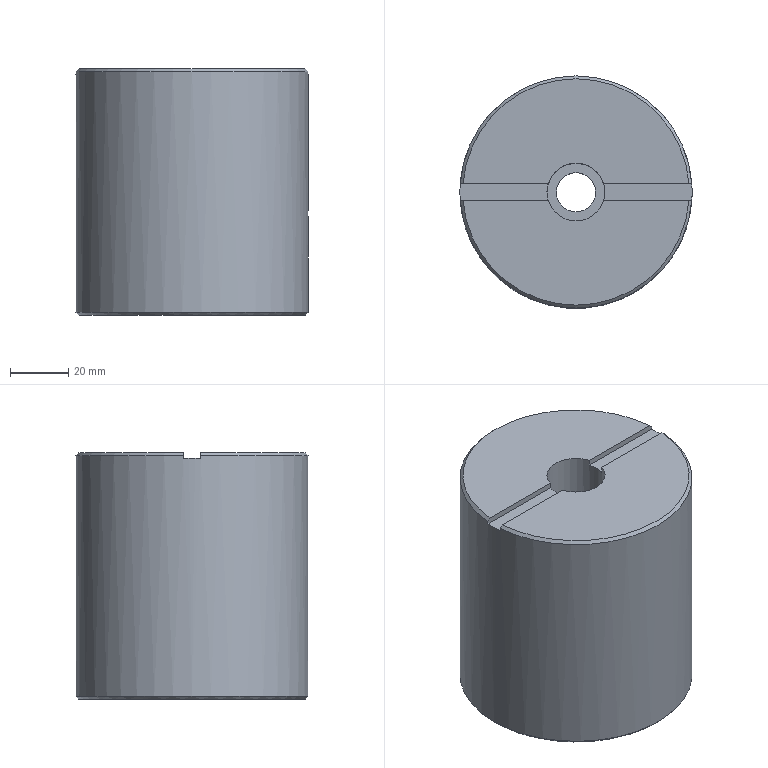Part | STEP file | 008_id4090_x_t | 1 solid | 18 faces | box 80 x 80 x 85 mm | volume 404567 mm3 | plane 11 | cylinder 4 | cone 3 | commonest cylinder face diameters 3.4 x1 13.509 x1 20.008 x1 80 x1
STEP:
#1=CARTESIAN_POINT('',(3931.979,552.,5.));
#2=VERTEX_POINT('',#1);
#3=CARTESIAN_POINT('',(3961.32,552.,5.));
#4=VERTEX_POINT('',#3);
#5=CARTESIAN_POINT('',(3873.935,552.,5.));
#6=DIRECTION('',(1.,0.,0.));
#7=VECTOR('',#6,1.);
#8=LINE('',#5,#7);
#9=EDGE_CURVE('',#2,#4,#8,.T.);
#10=ORIENTED_EDGE('',*,*,#9,.F.);
#11=CARTESIAN_POINT('',(3912.892,552.,5.));
#12=VERTEX_POINT('',#11);
#13=CARTESIAN_POINT('',(3922.435,555.,5.));
#14=DIRECTION('',(0.,0.,-1.));
#15=DIRECTION('',(-1.,0.,0.));
#16=AXIS2_PLACEMENT_3D('',#13,#14,#15);
#17=CIRCLE('',#16,10.004);
#18=EDGE_CURVE('',#2,#12,#17,.T.);
#19=ORIENTED_EDGE('',*,*,#18,.T.);
#20=CARTESIAN_POINT('',(3883.551,552.,5.));
#21=VERTEX_POINT('',#20);
#22=CARTESIAN_POINT('',(3873.935,552.,5.));
#23=DIRECTION('',(1.,0.,0.));
#24=VECTOR('',#23,1.);
#25=LINE('',#22,#24);
#26=EDGE_CURVE('',#21,#12,#25,.T.);
#27=ORIENTED_EDGE('',*,*,#26,.F.);
#28=CARTESIAN_POINT('',(3922.435,555.,5.));
#29=DIRECTION('',(0.,0.,-1.));
#30=DIRECTION('',(1.,0.,0.));
#31=AXIS2_PLACEMENT_3D('',#28,#29,#30);
#32=CIRCLE('',#31,39.);
#33=EDGE_CURVE('',#4,#21,#32,.T.);
#34=ORIENTED_EDGE('',*,*,#33,.F.);
#35=EDGE_LOOP('',(#10,#19,#27,#34));
#36=FACE_OUTER_BOUND('',#35,.T.);
#37=CARTESIAN_POINT('',(3922.435,555.,5.));
#38=DIRECTION('',(0.,0.,1.));
#39=DIRECTION('',(1.,0.,0.));
#40=AXIS2_PLACEMENT_3D('',#37,#38,#39);
#41=PLANE('',#40);
#42=ADVANCED_FACE('',(#36),#41,.T.);
#43=CARTESIAN_POINT('',(3883.551,558.,5.));
#44=VERTEX_POINT('',#43);
#45=CARTESIAN_POINT('',(3912.892,558.,5.));
#46=VERTEX_POINT('',#45);
#47=CARTESIAN_POINT('',(3922.435,558.,5.));
#48=DIRECTION('',(1.,0.,0.));
#49=VECTOR('',#48,1.);
#50=LINE('',#47,#49);
#51=EDGE_CURVE('',#44,#46,#50,.T.);
#52=ORIENTED_EDGE('',*,*,#51,.T.);
#53=CARTESIAN_POINT('',(3931.979,558.,5.));
#54=VERTEX_POINT('',#53);
#55=CARTESIAN_POINT('',(3922.435,555.,5.));
#56=DIRECTION('',(0.,0.,-1.));
#57=DIRECTION('',(-1.,0.,0.));
#58=AXIS2_PLACEMENT_3D('',#55,#56,#57);
#59=CIRCLE('',#58,10.004);
#60=EDGE_CURVE('',#46,#54,#59,.T.);
#61=ORIENTED_EDGE('',*,*,#60,.T.);
#62=CARTESIAN_POINT('',(3961.32,558.,5.));
#63=VERTEX_POINT('',#62);
#64=CARTESIAN_POINT('',(3922.435,558.,5.));
#65=DIRECTION('',(1.,0.,0.));
#66=VECTOR('',#65,1.);
#67=LINE('',#64,#66);
#68=EDGE_CURVE('',#54,#63,#67,.T.);
#69=ORIENTED_EDGE('',*,*,#68,.T.);
#70=CARTESIAN_POINT('',(3922.435,555.,5.));
#71=DIRECTION('',(0.,0.,-1.));
#72=DIRECTION('',(1.,0.,0.));
#73=AXIS2_PLACEMENT_3D('',#70,#71,#72);
#74=CIRCLE('',#73,39.);
#75=EDGE_CURVE('',#44,#63,#74,.T.);
#76=ORIENTED_EDGE('',*,*,#75,.F.);
#77=EDGE_LOOP('',(#52,#61,#69,#76));
#78=FACE_OUTER_BOUND('',#77,.T.);
#79=CARTESIAN_POINT('',(3922.435,555.,5.));
#80=DIRECTION('',(0.,0.,1.));
#81=DIRECTION('',(1.,0.,0.));
#82=AXIS2_PLACEMENT_3D('',#79,#80,#81);
#83=PLANE('',#82);
#84=ADVANCED_FACE('',(#78),#83,.T.);
#85=CARTESIAN_POINT('',(3962.435,555.,-79.));
#86=VERTEX_POINT('',#85);
#87=CARTESIAN_POINT('',(3922.435,555.,-79.));
#88=DIRECTION('',(0.,0.,-1.));
#89=DIRECTION('',(1.,0.,0.));
#90=AXIS2_PLACEMENT_3D('',#87,#88,#89);
#91=CIRCLE('',#90,40.);
#92=EDGE_CURVE('',#86,#86,#91,.T.);
#93=ORIENTED_EDGE('',*,*,#92,.F.);
#94=EDGE_LOOP('',(#93));
#95=FACE_BOUND('',#94,.T.);
#96=CARTESIAN_POINT('',(3882.548,552.,3.));
#97=VERTEX_POINT('',#96);
#98=CARTESIAN_POINT('',(3882.548,552.,4.));
#99=VERTEX_POINT('',#98);
#100=CARTESIAN_POINT('',(3882.548,552.,-80.));
#101=DIRECTION('',(0.,0.,1.));
#102=VECTOR('',#101,1.);
#103=LINE('',#100,#102);
#104=EDGE_CURVE('',#97,#99,#103,.T.);
#105=ORIENTED_EDGE('',*,*,#104,.F.);
#106=CARTESIAN_POINT('',(3882.548,558.,3.));
#107=VERTEX_POINT('',#106);
#108=CARTESIAN_POINT('',(3922.435,555.,3.));
#109=DIRECTION('',(0.,0.,1.));
#110=DIRECTION('',(-1.,0.,0.));
#111=AXIS2_PLACEMENT_3D('',#108,#109,#110);
#112=CIRCLE('',#111,40.);
#113=EDGE_CURVE('',#107,#97,#112,.T.);
#114=ORIENTED_EDGE('',*,*,#113,.F.);
#115=CARTESIAN_POINT('',(3882.548,558.,4.));
#116=VERTEX_POINT('',#115);
#117=CARTESIAN_POINT('',(3882.548,558.,-80.));
#118=DIRECTION('',(0.,0.,-1.));
#119=VECTOR('',#118,1.);
#120=LINE('',#117,#119);
#121=EDGE_CURVE('',#116,#107,#120,.T.);
#122=ORIENTED_EDGE('',*,*,#121,.F.);
#123=CARTESIAN_POINT('',(3962.323,558.,4.));
#124=VERTEX_POINT('',#123);
#125=CARTESIAN_POINT('',(3922.435,555.,4.));
#126=DIRECTION('',(0.,0.,1.));
#127=DIRECTION('',(1.,0.,0.));
#128=AXIS2_PLACEMENT_3D('',#125,#126,#127);
#129=CIRCLE('',#128,40.);
#130=EDGE_CURVE('',#124,#116,#129,.T.);
#131=ORIENTED_EDGE('',*,*,#130,.F.);
#132=CARTESIAN_POINT('',(3962.323,558.,3.));
#133=VERTEX_POINT('',#132);
#134=CARTESIAN_POINT('',(3962.323,558.,-80.));
#135=DIRECTION('',(0.,0.,1.));
#136=VECTOR('',#135,1.);
#137=LINE('',#134,#136);
#138=EDGE_CURVE('',#133,#124,#137,.T.);
#139=ORIENTED_EDGE('',*,*,#138,.F.);
#140=CARTESIAN_POINT('',(3962.323,552.,3.));
#141=VERTEX_POINT('',#140);
#142=CARTESIAN_POINT('',(3922.435,555.,3.));
#143=DIRECTION('',(0.,0.,1.));
#144=DIRECTION('',(-1.,0.,0.));
#145=AXIS2_PLACEMENT_3D('',#142,#143,#144);
#146=CIRCLE('',#145,40.);
#147=EDGE_CURVE('',#141,#133,#146,.T.);
#148=ORIENTED_EDGE('',*,*,#147,.F.);
#149=CARTESIAN_POINT('',(3962.323,552.,4.));
#150=VERTEX_POINT('',#149);
#151=CARTESIAN_POINT('',(3962.323,552.,-80.));
#152=DIRECTION('',(0.,0.,-1.));
#153=VECTOR('',#152,1.);
#154=LINE('',#151,#153);
#155=EDGE_CURVE('',#150,#141,#154,.T.);
#156=ORIENTED_EDGE('',*,*,#155,.F.);
#157=CARTESIAN_POINT('',(3922.435,555.,4.));
#158=DIRECTION('',(0.,0.,1.));
#159=DIRECTION('',(1.,0.,0.));
#160=AXIS2_PLACEMENT_3D('',#157,#158,#159);
#161=CIRCLE('',#160,40.);
#162=EDGE_CURVE('',#99,#150,#161,.T.);
#163=ORIENTED_EDGE('',*,*,#162,.F.);
#164=EDGE_LOOP('',(#105,#114,#122,#131,#139,#148,#156,#163));
#165=FACE_BOUND('',#164,.T.);
#166=CARTESIAN_POINT('',(3962.435,555.182,-43.31));
#167=VERTEX_POINT('',#166);
#168=CARTESIAN_POINT('',(3962.435,555.182,-43.31));
#169=CARTESIAN_POINT('',(3962.436,554.993,-43.289));
#170=CARTESIAN_POINT('',(3962.435,554.798,-43.301));
#171=CARTESIAN_POINT('',(3962.433,554.613,-43.345));
#172=CARTESIAN_POINT('',(3962.432,554.427,-43.388));
#173=CARTESIAN_POINT('',(3962.428,554.247,-43.464));
#174=CARTESIAN_POINT('',(3962.425,554.087,-43.566));
#175=CARTESIAN_POINT('',(3962.421,553.926,-43.668));
#176=CARTESIAN_POINT('',(3962.417,553.781,-43.799));
#177=CARTESIAN_POINT('',(3962.413,553.664,-43.949));
#178=CARTESIAN_POINT('',(3962.409,553.546,-44.099));
#179=CARTESIAN_POINT('',(3962.405,553.453,-44.271));
#180=CARTESIAN_POINT('',(3962.403,553.391,-44.451));
#181=CARTESIAN_POINT('',(3962.4,553.33,-44.631));
#182=CARTESIAN_POINT('',(3962.399,553.298,-44.824));
#183=CARTESIAN_POINT('',(3962.399,553.3,-45.014));
#184=CARTESIAN_POINT('',(3962.399,553.302,-45.204));
#185=CARTESIAN_POINT('',(3962.401,553.336,-45.397));
#186=CARTESIAN_POINT('',(3962.403,553.4,-45.576));
#187=CARTESIAN_POINT('',(3962.406,553.465,-45.755));
#188=CARTESIAN_POINT('',(3962.41,553.561,-45.925));
#189=CARTESIAN_POINT('',(3962.413,553.681,-46.072));
#190=CARTESIAN_POINT('',(3962.417,553.801,-46.22));
#191=CARTESIAN_POINT('',(3962.422,553.948,-46.349));
#192=CARTESIAN_POINT('',(3962.425,554.11,-46.448));
#193=CARTESIAN_POINT('',(3962.429,554.272,-46.548));
#194=CARTESIAN_POINT('',(3962.432,554.454,-46.621));
#195=CARTESIAN_POINT('',(3962.434,554.64,-46.661));
#196=CARTESIAN_POINT('',(3962.435,554.826,-46.702));
#197=CARTESIAN_POINT('',(3962.436,555.021,-46.71));
#198=CARTESIAN_POINT('',(3962.435,555.21,-46.687));
#199=CARTESIAN_POINT('',(3962.434,555.399,-46.664));
#200=CARTESIAN_POINT('',(3962.431,555.586,-46.607));
#201=CARTESIAN_POINT('',(3962.428,555.756,-46.523));
#202=CARTESIAN_POINT('',(3962.425,555.926,-46.438));
#203=CARTESIAN_POINT('',(3962.421,556.084,-46.323));
#204=CARTESIAN_POINT('',(3962.417,556.217,-46.187));
#205=CARTESIAN_POINT('',(3962.413,556.35,-46.051));
#206=CARTESIAN_POINT('',(3962.409,556.461,-45.89));
#207=CARTESIAN_POINT('',(3962.406,556.541,-45.717));
#208=CARTESIAN_POINT('',(3962.402,556.622,-45.545));
#209=CARTESIAN_POINT('',(3962.4,556.673,-45.356));
#210=CARTESIAN_POINT('',(3962.399,556.692,-45.166));
#211=CARTESIAN_POINT('',(3962.399,556.71,-44.977));
#212=CARTESIAN_POINT('',(3962.399,556.697,-44.782));
#213=CARTESIAN_POINT('',(3962.401,556.652,-44.597));
#214=CARTESIAN_POINT('',(3962.403,556.607,-44.413));
#215=CARTESIAN_POINT('',(3962.406,556.529,-44.233));
#216=CARTESIAN_POINT('',(3962.41,556.425,-44.074));
#217=CARTESIAN_POINT('',(3962.414,556.322,-43.914));
#218=CARTESIAN_POINT('',(3962.418,556.189,-43.77));
#219=CARTESIAN_POINT('',(3962.422,556.039,-43.654));
#220=CARTESIAN_POINT('',(3962.426,555.888,-43.538));
#221=CARTESIAN_POINT('',(3962.429,555.715,-43.446));
#222=CARTESIAN_POINT('',(3962.432,555.535,-43.386));
#223=CARTESIAN_POINT('',(3962.433,555.42,-43.348));
#224=CARTESIAN_POINT('',(3962.434,555.301,-43.323));
#225=CARTESIAN_POINT('',(3962.435,555.182,-43.31));
#226=B_SPLINE_CURVE_WITH_KNOTS('',3,(#168,#169,#170,#171,#172,#173,#174,#175,#176,#177,#178,#179,#180,#181,#182,#183,#184,#185,#186,#187,#188,#189,#190,#191,#192,#193,#194,#195,#196,#197,#198,#199,#200,#201,#202,#203,#204,#205,#206,#207,#208,#209,#210,#211,#212,#213,#214,#215,#216,#217,#218,#219,#220,#221,#222,#223,#224,#225),.UNSPECIFIED.,.T.,.F.,(1,3,3,3,3,3,3,3,3,3,3,3,3,3,3,3,3,3,3,3,3,1),(-0.03366,0.,0.05366,0.1073,0.161,0.2147,0.2684,0.3221,0.3757,0.4295,0.4832,0.5369,0.5905,0.6442,0.6979,0.7516,0.8053,0.8589,0.9126,0.9663,1.,1.054),.UNSPECIFIED.);
#227=EDGE_CURVE('',#167,#167,#226,.T.);
#228=ORIENTED_EDGE('',*,*,#227,.F.);
#229=EDGE_LOOP('',(#228));
#230=FACE_BOUND('',#229,.T.);
#231=CARTESIAN_POINT('',(3922.435,555.,-80.));
#232=DIRECTION('',(0.,0.,1.));
#233=DIRECTION('',(1.,0.,0.));
#234=AXIS2_PLACEMENT_3D('',#231,#232,#233);
#235=CYLINDRICAL_SURFACE('',#234,40.);
#236=ADVANCED_FACE('',(#95,#165,#230),#235,.T.);
#237=CARTESIAN_POINT('',(3915.681,555.,-80.));
#238=VERTEX_POINT('',#237);
#239=CARTESIAN_POINT('',(3922.435,555.,-80.));
#240=DIRECTION('',(0.,0.,1.));
#241=DIRECTION('',(-1.,0.,0.));
#242=AXIS2_PLACEMENT_3D('',#239,#240,#241);
#243=CIRCLE('',#242,6.755);
#244=EDGE_CURVE('',#238,#238,#243,.T.);
#245=ORIENTED_EDGE('',*,*,#244,.T.);
#246=EDGE_LOOP('',(#245));
#247=FACE_BOUND('',#246,.T.);
#248=CARTESIAN_POINT('',(3961.435,555.,-80.));
#249=VERTEX_POINT('',#248);
#250=CARTESIAN_POINT('',(3922.435,555.,-80.));
#251=DIRECTION('',(0.,0.,1.));
#252=DIRECTION('',(1.,0.,0.));
#253=AXIS2_PLACEMENT_3D('',#250,#251,#252);
#254=CIRCLE('',#253,39.);
#255=EDGE_CURVE('',#249,#249,#254,.T.);
#256=ORIENTED_EDGE('',*,*,#255,.F.);
#257=EDGE_LOOP('',(#256));
#258=FACE_BOUND('',#257,.T.);
#259=CARTESIAN_POINT('',(3922.435,555.,-80.));
#260=DIRECTION('',(0.,0.,1.));
#261=DIRECTION('',(1.,0.,0.));
#262=AXIS2_PLACEMENT_3D('',#259,#260,#261);
#263=PLANE('',#262);
#264=ADVANCED_FACE('',(#247,#258),#263,.F.);
#265=CARTESIAN_POINT('',(3912.892,552.,3.));
#266=VERTEX_POINT('',#265);
#267=CARTESIAN_POINT('',(3912.892,552.,5.));
#268=DIRECTION('',(0.,0.,1.));
#269=VECTOR('',#268,1.);
#270=LINE('',#267,#269);
#271=EDGE_CURVE('',#266,#12,#270,.T.);
#272=ORIENTED_EDGE('',*,*,#271,.F.);
#273=CARTESIAN_POINT('',(3873.935,552.,3.));
#274=DIRECTION('',(1.,0.,0.));
#275=VECTOR('',#274,1.);
#276=LINE('',#273,#275);
#277=EDGE_CURVE('',#97,#266,#276,.T.);
#278=ORIENTED_EDGE('',*,*,#277,.F.);
#279=ORIENTED_EDGE('',*,*,#104,.T.);
#280=CARTESIAN_POINT('',(3883.551,552.,5.));
#281=CARTESIAN_POINT('',(3883.45,552.,4.9));
#282=CARTESIAN_POINT('',(3883.35,552.,4.8));
#283=CARTESIAN_POINT('',(3883.016,552.,4.467));
#284=CARTESIAN_POINT('',(3882.782,552.,4.233));
#285=CARTESIAN_POINT('',(3882.548,552.,4.));
#286=B_SPLINE_CURVE_WITH_KNOTS('',3,(#280,#281,#282,#283,#284,#285),.UNSPECIFIED.,.F.,.F.,(4,2,4),(0.,0.3001,1.),.UNSPECIFIED.);
#287=EDGE_CURVE('',#21,#99,#286,.T.);
#288=ORIENTED_EDGE('',*,*,#287,.F.);
#289=ORIENTED_EDGE('',*,*,#26,.T.);
#290=EDGE_LOOP('',(#272,#278,#279,#288,#289));
#291=FACE_OUTER_BOUND('',#290,.T.);
#292=CARTESIAN_POINT('',(3873.935,552.,5.));
#293=DIRECTION('',(0.,1.,0.));
#294=DIRECTION('',(0.,0.,-1.));
#295=AXIS2_PLACEMENT_3D('',#292,#293,#294);
#296=PLANE('',#295);
#297=ADVANCED_FACE('',(#291),#296,.T.);
#298=CARTESIAN_POINT('',(3912.892,558.,3.));
#299=VERTEX_POINT('',#298);
#300=CARTESIAN_POINT('',(3922.435,555.,3.));
#301=DIRECTION('',(0.,0.,1.));
#302=DIRECTION('',(-1.,0.,0.));
#303=AXIS2_PLACEMENT_3D('',#300,#301,#302);
#304=CIRCLE('',#303,10.004);
#305=EDGE_CURVE('',#299,#266,#304,.T.);
#306=ORIENTED_EDGE('',*,*,#305,.F.);
#307=CARTESIAN_POINT('',(3922.435,558.,3.));
#308=DIRECTION('',(1.,0.,0.));
#309=VECTOR('',#308,1.);
#310=LINE('',#307,#309);
#311=EDGE_CURVE('',#107,#299,#310,.T.);
#312=ORIENTED_EDGE('',*,*,#311,.F.);
#313=ORIENTED_EDGE('',*,*,#113,.T.);
#314=ORIENTED_EDGE('',*,*,#277,.T.);
#315=EDGE_LOOP('',(#306,#312,#313,#314));
#316=FACE_OUTER_BOUND('',#315,.T.);
#317=CARTESIAN_POINT('',(3922.435,555.,3.));
#318=DIRECTION('',(0.,0.,1.));
#319=DIRECTION('',(1.,0.,0.));
#320=AXIS2_PLACEMENT_3D('',#317,#318,#319);
#321=PLANE('',#320);
#322=ADVANCED_FACE('',(#316),#321,.T.);
#323=CARTESIAN_POINT('',(3912.892,558.,5.));
#324=DIRECTION('',(0.,0.,-1.));
#325=VECTOR('',#324,1.);
#326=LINE('',#323,#325);
#327=EDGE_CURVE('',#46,#299,#326,.T.);
#328=ORIENTED_EDGE('',*,*,#327,.F.);
#329=ORIENTED_EDGE('',*,*,#51,.F.);
#330=CARTESIAN_POINT('',(3882.548,558.,4.));
#331=CARTESIAN_POINT('',(3882.782,558.,4.233));
#332=CARTESIAN_POINT('',(3883.016,558.,4.467));
#333=CARTESIAN_POINT('',(3883.35,558.,4.8));
#334=CARTESIAN_POINT('',(3883.45,558.,4.9));
#335=CARTESIAN_POINT('',(3883.551,558.,5.));
#336=B_SPLINE_CURVE_WITH_KNOTS('',3,(#330,#331,#332,#333,#334,#335),.UNSPECIFIED.,.F.,.F.,(4,2,4),(0.,0.6999,1.),.UNSPECIFIED.);
#337=EDGE_CURVE('',#116,#44,#336,.T.);
#338=ORIENTED_EDGE('',*,*,#337,.F.);
#339=ORIENTED_EDGE('',*,*,#121,.T.);
#340=ORIENTED_EDGE('',*,*,#311,.T.);
#341=EDGE_LOOP('',(#328,#329,#338,#339,#340));
#342=FACE_OUTER_BOUND('',#341,.T.);
#343=CARTESIAN_POINT('',(3873.935,558.,3.73));
#344=DIRECTION('',(0.,-1.,0.));
#345=DIRECTION('',(0.,0.,1.));
#346=AXIS2_PLACEMENT_3D('',#343,#344,#345);
#347=PLANE('',#346);
#348=ADVANCED_FACE('',(#342),#347,.T.);
#349=CARTESIAN_POINT('',(3931.979,552.,3.));
#350=VERTEX_POINT('',#349);
#351=CARTESIAN_POINT('',(3931.979,558.,3.));
#352=VERTEX_POINT('',#351);
#353=CARTESIAN_POINT('',(3922.435,555.,3.));
#354=DIRECTION('',(0.,0.,1.));
#355=DIRECTION('',(-1.,0.,0.));
#356=AXIS2_PLACEMENT_3D('',#353,#354,#355);
#357=CIRCLE('',#356,10.004);
#358=EDGE_CURVE('',#350,#352,#357,.T.);
#359=ORIENTED_EDGE('',*,*,#358,.F.);
#360=CARTESIAN_POINT('',(3873.935,552.,3.));
#361=DIRECTION('',(1.,0.,0.));
#362=VECTOR('',#361,1.);
#363=LINE('',#360,#362);
#364=EDGE_CURVE('',#350,#141,#363,.T.);
#365=ORIENTED_EDGE('',*,*,#364,.T.);
#366=ORIENTED_EDGE('',*,*,#147,.T.);
#367=CARTESIAN_POINT('',(3922.435,558.,3.));
#368=DIRECTION('',(1.,0.,0.));
#369=VECTOR('',#368,1.);
#370=LINE('',#367,#369);
#371=EDGE_CURVE('',#352,#133,#370,.T.);
#372=ORIENTED_EDGE('',*,*,#371,.F.);
#373=EDGE_LOOP('',(#359,#365,#366,#372));
#374=FACE_OUTER_BOUND('',#373,.T.);
#375=CARTESIAN_POINT('',(3922.435,555.,3.));
#376=DIRECTION('',(0.,0.,1.));
#377=DIRECTION('',(1.,0.,0.));
#378=AXIS2_PLACEMENT_3D('',#375,#376,#377);
#379=PLANE('',#378);
#380=ADVANCED_FACE('',(#374),#379,.T.);
#381=CARTESIAN_POINT('',(3931.979,552.,5.));
#382=DIRECTION('',(0.,0.,-1.));
#383=VECTOR('',#382,1.);
#384=LINE('',#381,#383);
#385=EDGE_CURVE('',#2,#350,#384,.T.);
#386=ORIENTED_EDGE('',*,*,#385,.F.);
#387=ORIENTED_EDGE('',*,*,#9,.T.);
#388=CARTESIAN_POINT('',(3962.323,552.,4.));
#389=CARTESIAN_POINT('',(3962.089,552.,4.233));
#390=CARTESIAN_POINT('',(3961.855,552.,4.467));
#391=CARTESIAN_POINT('',(3961.52,552.,4.8));
#392=CARTESIAN_POINT('',(3961.42,552.,4.9));
#393=CARTESIAN_POINT('',(3961.32,552.,5.));
#394=B_SPLINE_CURVE_WITH_KNOTS('',3,(#388,#389,#390,#391,#392,#393),.UNSPECIFIED.,.F.,.F.,(4,2,4),(0.,0.6999,1.),.UNSPECIFIED.);
#395=EDGE_CURVE('',#150,#4,#394,.T.);
#396=ORIENTED_EDGE('',*,*,#395,.F.);
#397=ORIENTED_EDGE('',*,*,#155,.T.);
#398=ORIENTED_EDGE('',*,*,#364,.F.);
#399=EDGE_LOOP('',(#386,#387,#396,#397,#398));
#400=FACE_OUTER_BOUND('',#399,.T.);
#401=CARTESIAN_POINT('',(3873.935,552.,5.));
#402=DIRECTION('',(0.,1.,0.));
#403=DIRECTION('',(0.,0.,-1.));
#404=AXIS2_PLACEMENT_3D('',#401,#402,#403);
#405=PLANE('',#404);
#406=ADVANCED_FACE('',(#400),#405,.T.);
#407=CARTESIAN_POINT('',(3931.979,558.,5.));
#408=DIRECTION('',(0.,0.,1.));
#409=VECTOR('',#408,1.);
#410=LINE('',#407,#409);
#411=EDGE_CURVE('',#352,#54,#410,.T.);
#412=ORIENTED_EDGE('',*,*,#411,.F.);
#413=ORIENTED_EDGE('',*,*,#371,.T.);
#414=ORIENTED_EDGE('',*,*,#138,.T.);
#415=CARTESIAN_POINT('',(3961.32,558.,5.));
#416=CARTESIAN_POINT('',(3961.42,558.,4.9));
#417=CARTESIAN_POINT('',(3961.52,558.,4.8));
#418=CARTESIAN_POINT('',(3961.855,558.,4.467));
#419=CARTESIAN_POINT('',(3962.089,558.,4.233));
#420=CARTESIAN_POINT('',(3962.323,558.,4.));
#421=B_SPLINE_CURVE_WITH_KNOTS('',3,(#415,#416,#417,#418,#419,#420),.UNSPECIFIED.,.F.,.F.,(4,2,4),(0.,0.3001,1.),.UNSPECIFIED.);
#422=EDGE_CURVE('',#63,#124,#421,.T.);
#423=ORIENTED_EDGE('',*,*,#422,.F.);
#424=ORIENTED_EDGE('',*,*,#68,.F.);
#425=EDGE_LOOP('',(#412,#413,#414,#423,#424));
#426=FACE_OUTER_BOUND('',#425,.T.);
#427=CARTESIAN_POINT('',(3873.935,558.,3.73));
#428=DIRECTION('',(0.,-1.,0.));
#429=DIRECTION('',(0.,0.,1.));
#430=AXIS2_PLACEMENT_3D('',#427,#428,#429);
#431=PLANE('',#430);
#432=ADVANCED_FACE('',(#426),#431,.T.);
#433=ORIENTED_EDGE('',*,*,#227,.T.);
#434=EDGE_LOOP('',(#433));
#435=FACE_BOUND('',#434,.T.);
#436=CARTESIAN_POINT('',(3947.935,556.7,-45.));
#437=VERTEX_POINT('',#436);
#438=CARTESIAN_POINT('',(3947.935,555.,-45.));
#439=DIRECTION('',(-1.,0.,0.));
#440=DIRECTION('',(0.,1.,0.));
#441=AXIS2_PLACEMENT_3D('',#438,#439,#440);
#442=CIRCLE('',#441,1.7);
#443=EDGE_CURVE('',#437,#437,#442,.T.);
#444=ORIENTED_EDGE('',*,*,#443,.T.);
#445=EDGE_LOOP('',(#444));
#446=FACE_BOUND('',#445,.T.);
#447=CARTESIAN_POINT('',(3947.935,555.,-45.));
#448=DIRECTION('',(1.,0.,0.));
#449=DIRECTION('',(0.,-1.,0.));
#450=AXIS2_PLACEMENT_3D('',#447,#448,#449);
#451=CYLINDRICAL_SURFACE('',#450,1.7);
#452=ADVANCED_FACE('',(#435,#446),#451,.F.);
#453=ORIENTED_EDGE('',*,*,#443,.F.);
#454=EDGE_LOOP('',(#453));
#455=FACE_OUTER_BOUND('',#454,.T.);
#456=CARTESIAN_POINT('',(3947.935,555.,-45.));
#457=DIRECTION('',(-1.,0.,0.));
#458=DIRECTION('',(0.,1.,0.));
#459=AXIS2_PLACEMENT_3D('',#456,#457,#458);
#460=PLANE('',#459);
#461=ADVANCED_FACE('',(#455),#460,.F.);
#462=ORIENTED_EDGE('',*,*,#395,.T.);
#463=ORIENTED_EDGE('',*,*,#33,.T.);
#464=ORIENTED_EDGE('',*,*,#287,.T.);
#465=ORIENTED_EDGE('',*,*,#162,.T.);
#466=EDGE_LOOP('',(#462,#463,#464,#465));
#467=FACE_OUTER_BOUND('',#466,.T.);
#468=CARTESIAN_POINT('',(3922.435,555.,5.));
#469=DIRECTION('',(0.,0.,-1.));
#470=DIRECTION('',(-1.,0.,0.));
#471=AXIS2_PLACEMENT_3D('',#468,#469,#470);
#472=CONICAL_SURFACE('',#471,39.,45.);
#473=ADVANCED_FACE('',(#467),#472,.T.);
#474=ORIENTED_EDGE('',*,*,#337,.T.);
#475=ORIENTED_EDGE('',*,*,#75,.T.);
#476=ORIENTED_EDGE('',*,*,#422,.T.);
#477=ORIENTED_EDGE('',*,*,#130,.T.);
#478=EDGE_LOOP('',(#474,#475,#476,#477));
#479=FACE_OUTER_BOUND('',#478,.T.);
#480=CARTESIAN_POINT('',(3922.435,555.,5.));
#481=DIRECTION('',(0.,0.,-1.));
#482=DIRECTION('',(-1.,0.,0.));
#483=AXIS2_PLACEMENT_3D('',#480,#481,#482);
#484=CONICAL_SURFACE('',#483,39.,45.);
#485=ADVANCED_FACE('',(#479),#484,.T.);
#486=ORIENTED_EDGE('',*,*,#255,.T.);
#487=EDGE_LOOP('',(#486));
#488=FACE_BOUND('',#487,.T.);
#489=ORIENTED_EDGE('',*,*,#92,.T.);
#490=EDGE_LOOP('',(#489));
#491=FACE_BOUND('',#490,.T.);
#492=CARTESIAN_POINT('',(3922.435,555.,-79.));
#493=DIRECTION('',(0.,0.,1.));
#494=DIRECTION('',(1.,0.,0.));
#495=AXIS2_PLACEMENT_3D('',#492,#493,#494);
#496=CONICAL_SURFACE('',#495,40.,45.);
#497=ADVANCED_FACE('',(#488,#491),#496,.T.);
#498=CARTESIAN_POINT('',(3929.19,555.,-50.));
#499=VERTEX_POINT('',#498);
#500=CARTESIAN_POINT('',(3922.435,555.,-50.));
#501=DIRECTION('',(0.,0.,-1.));
#502=DIRECTION('',(1.,0.,0.));
#503=AXIS2_PLACEMENT_3D('',#500,#501,#502);
#504=CIRCLE('',#503,6.755);
#505=EDGE_CURVE('',#499,#499,#504,.T.);
#506=ORIENTED_EDGE('',*,*,#505,.F.);
#507=EDGE_LOOP('',(#506));
#508=FACE_BOUND('',#507,.T.);
#509=ORIENTED_EDGE('',*,*,#244,.F.);
#510=EDGE_LOOP('',(#509));
#511=FACE_BOUND('',#510,.T.);
#512=CARTESIAN_POINT('',(3922.435,555.,5.));
#513=DIRECTION('',(0.,0.,-1.));
#514=DIRECTION('',(-1.,0.,0.));
#515=AXIS2_PLACEMENT_3D('',#512,#513,#514);
#516=CYLINDRICAL_SURFACE('',#515,6.755);
#517=ADVANCED_FACE('',(#508,#511),#516,.F.);
#518=ORIENTED_EDGE('',*,*,#505,.T.);
#519=EDGE_LOOP('',(#518));
#520=FACE_BOUND('',#519,.T.);
#521=CARTESIAN_POINT('',(3912.431,555.,-50.));
#522=VERTEX_POINT('',#521);
#523=CARTESIAN_POINT('',(3922.435,555.,-50.));
#524=DIRECTION('',(0.,0.,-1.));
#525=DIRECTION('',(-1.,0.,0.));
#526=AXIS2_PLACEMENT_3D('',#523,#524,#525);
#527=CIRCLE('',#526,10.004);
#528=EDGE_CURVE('',#522,#522,#527,.T.);
#529=ORIENTED_EDGE('',*,*,#528,.F.);
#530=EDGE_LOOP('',(#529));
#531=FACE_BOUND('',#530,.T.);
#532=CARTESIAN_POINT('',(3922.435,555.,-50.));
#533=DIRECTION('',(0.,0.,-1.));
#534=DIRECTION('',(1.,0.,0.));
#535=AXIS2_PLACEMENT_3D('',#532,#533,#534);
#536=PLANE('',#535);
#537=ADVANCED_FACE('',(#520,#531),#536,.F.);
#538=ORIENTED_EDGE('',*,*,#271,.T.);
#539=ORIENTED_EDGE('',*,*,#18,.F.);
#540=ORIENTED_EDGE('',*,*,#385,.T.);
#541=ORIENTED_EDGE('',*,*,#358,.T.);
#542=ORIENTED_EDGE('',*,*,#411,.T.);
#543=ORIENTED_EDGE('',*,*,#60,.F.);
#544=ORIENTED_EDGE('',*,*,#327,.T.);
#545=ORIENTED_EDGE('',*,*,#305,.T.);
#546=EDGE_LOOP('',(#538,#539,#540,#541,#542,#543,#544,#545));
#547=FACE_BOUND('',#546,.T.);
#548=ORIENTED_EDGE('',*,*,#528,.T.);
#549=EDGE_LOOP('',(#548));
#550=FACE_BOUND('',#549,.T.);
#551=CARTESIAN_POINT('',(3922.435,555.,5.));
#552=DIRECTION('',(0.,0.,-1.));
#553=DIRECTION('',(-1.,0.,0.));
#554=AXIS2_PLACEMENT_3D('',#551,#552,#553);
#555=CYLINDRICAL_SURFACE('',#554,10.004);
#556=ADVANCED_FACE('',(#547,#550),#555,.F.);
#557=CLOSED_SHELL('',(#42,#84,#236,#264,#297,#322,#348,#380,#406,#432,#452,#461,#473,#485,#497,#517,#537,#556));
#558=MANIFOLD_SOLID_BREP('',#557);
#559=(LENGTH_UNIT()NAMED_UNIT(*)SI_UNIT(.MILLI.,.METRE.));
#560=UNCERTAINTY_MEASURE_WITH_UNIT(LENGTH_MEASURE(0.0508),#559,'','');
#561=(NAMED_UNIT(*)PLANE_ANGLE_UNIT()SI_UNIT($,.RADIAN.));
#562=PLANE_ANGLE_MEASURE_WITH_UNIT(PLANE_ANGLE_MEASURE(0.01745),#561);
#563=DIMENSIONAL_EXPONENTS(0.,0.,0.,0.,0.,0.,0.);
#564=(CONVERSION_BASED_UNIT('DEGREE',#562)NAMED_UNIT(#563)PLANE_ANGLE_UNIT());
#565=(NAMED_UNIT(*)SI_UNIT($,.STERADIAN.)SOLID_ANGLE_UNIT());
#566=(GEOMETRIC_REPRESENTATION_CONTEXT(3)GLOBAL_UNCERTAINTY_ASSIGNED_CONTEXT((#560))GLOBAL_UNIT_ASSIGNED_CONTEXT((#559,#564,#565))REPRESENTATION_CONTEXT('',''));
#567=ADVANCED_BREP_SHAPE_REPRESENTATION('',(#558),#566);